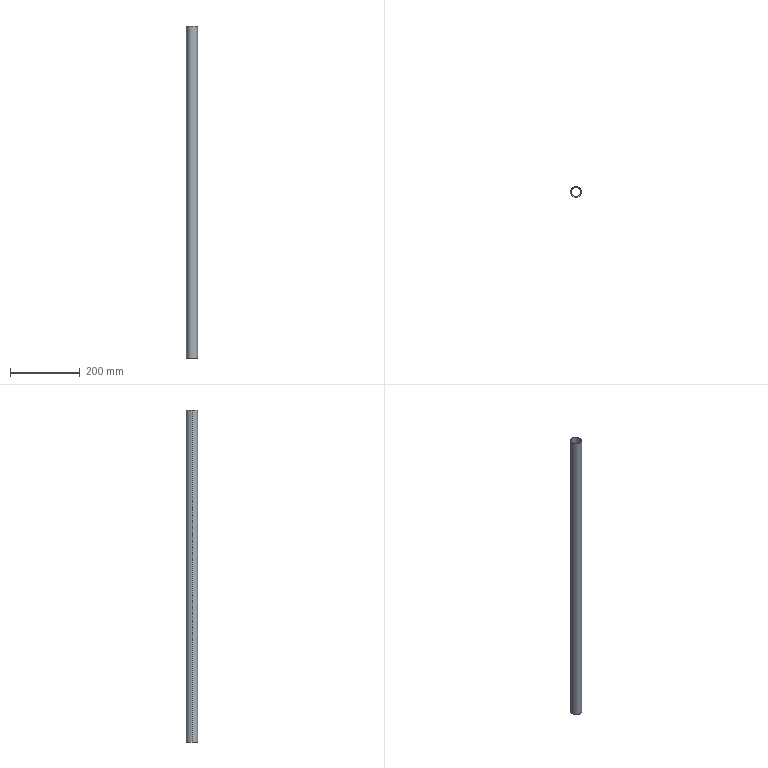Part | SolidWorks | features Extrusion 1 | 1 solid | 6 faces | box 32 x 32 x 950 mm | volume 179071 mm3 | cylinder 4 | plane 2 | commonest cylinder face diameters 28 x2 32 x2
STEP:
#1=CARTESIAN_POINT('',(-14.,0.,475.));
#2=VERTEX_POINT('',#1);
#3=CARTESIAN_POINT('',(14.,0.,475.));
#4=VERTEX_POINT('',#3);
#5=CARTESIAN_POINT('',(0.,0.,475.));
#6=DIRECTION('',(0.,0.,1.));
#7=DIRECTION('',(1.,0.,0.));
#8=AXIS2_PLACEMENT_3D('',#5,#6,#7);
#9=CIRCLE('',#8,14.);
#10=EDGE_CURVE('',#2,#4,#9,.T.);
#11=ORIENTED_EDGE('',*,*,#10,.T.);
#12=CARTESIAN_POINT('',(14.,0.,-475.));
#13=VERTEX_POINT('',#12);
#14=CARTESIAN_POINT('',(14.,0.,475.));
#15=DIRECTION('',(0.,0.,-1.));
#16=VECTOR('',#15,1000.);
#17=LINE('',#14,#16);
#18=EDGE_CURVE('',#4,#13,#17,.T.);
#19=ORIENTED_EDGE('',*,*,#18,.T.);
#20=CARTESIAN_POINT('',(-14.,0.,-475.));
#21=VERTEX_POINT('',#20);
#22=CARTESIAN_POINT('',(0.,0.,-475.));
#23=DIRECTION('',(0.,0.,1.));
#24=DIRECTION('',(1.,0.,0.));
#25=AXIS2_PLACEMENT_3D('',#22,#23,#24);
#26=CIRCLE('',#25,14.);
#27=EDGE_CURVE('',#21,#13,#26,.T.);
#28=ORIENTED_EDGE('',*,*,#27,.F.);
#29=CARTESIAN_POINT('',(-14.,0.,475.));
#30=DIRECTION('',(0.,0.,-1.));
#31=VECTOR('',#30,1000.);
#32=LINE('',#29,#31);
#33=EDGE_CURVE('',#2,#21,#32,.T.);
#34=ORIENTED_EDGE('',*,*,#33,.F.);
#35=EDGE_LOOP('',(#11,#19,#28,#34));
#36=FACE_OUTER_BOUND('',#35,.T.);
#37=CARTESIAN_POINT('',(0.,0.,475.));
#38=DIRECTION('',(0.,0.,-1.));
#39=DIRECTION('',(-1.,0.,0.));
#40=AXIS2_PLACEMENT_3D('',#37,#38,#39);
#41=CYLINDRICAL_SURFACE('',#40,14.);
#42=ADVANCED_FACE('',(#36),#41,.F.);
#43=CARTESIAN_POINT('',(16.,0.,475.));
#44=VERTEX_POINT('',#43);
#45=CARTESIAN_POINT('',(-16.,0.,475.));
#46=VERTEX_POINT('',#45);
#47=CARTESIAN_POINT('',(0.,0.,475.));
#48=DIRECTION('',(0.,0.,1.));
#49=DIRECTION('',(1.,0.,0.));
#50=AXIS2_PLACEMENT_3D('',#47,#48,#49);
#51=CIRCLE('',#50,16.);
#52=EDGE_CURVE('',#44,#46,#51,.T.);
#53=ORIENTED_EDGE('',*,*,#52,.F.);
#54=CARTESIAN_POINT('',(16.,0.,-475.));
#55=VERTEX_POINT('',#54);
#56=CARTESIAN_POINT('',(16.,0.,475.));
#57=DIRECTION('',(0.,0.,-1.));
#58=VECTOR('',#57,1000.);
#59=LINE('',#56,#58);
#60=EDGE_CURVE('',#44,#55,#59,.T.);
#61=ORIENTED_EDGE('',*,*,#60,.T.);
#62=CARTESIAN_POINT('',(-16.,0.,-475.));
#63=VERTEX_POINT('',#62);
#64=CARTESIAN_POINT('',(0.,0.,-475.));
#65=DIRECTION('',(0.,0.,1.));
#66=DIRECTION('',(1.,0.,0.));
#67=AXIS2_PLACEMENT_3D('',#64,#65,#66);
#68=CIRCLE('',#67,16.);
#69=EDGE_CURVE('',#55,#63,#68,.T.);
#70=ORIENTED_EDGE('',*,*,#69,.T.);
#71=CARTESIAN_POINT('',(-16.,0.,475.));
#72=DIRECTION('',(0.,0.,-1.));
#73=VECTOR('',#72,1000.);
#74=LINE('',#71,#73);
#75=EDGE_CURVE('',#46,#63,#74,.T.);
#76=ORIENTED_EDGE('',*,*,#75,.F.);
#77=EDGE_LOOP('',(#53,#61,#70,#76));
#78=FACE_OUTER_BOUND('',#77,.T.);
#79=CARTESIAN_POINT('',(0.,0.,475.));
#80=DIRECTION('',(0.,0.,-1.));
#81=DIRECTION('',(-1.,0.,0.));
#82=AXIS2_PLACEMENT_3D('',#79,#80,#81);
#83=CYLINDRICAL_SURFACE('',#82,16.);
#84=ADVANCED_FACE('',(#78),#83,.T.);
#85=CARTESIAN_POINT('',(0.,0.,475.));
#86=DIRECTION('',(0.,0.,1.));
#87=DIRECTION('',(1.,0.,0.));
#88=AXIS2_PLACEMENT_3D('',#85,#86,#87);
#89=CIRCLE('',#88,16.);
#90=EDGE_CURVE('',#46,#44,#89,.T.);
#91=ORIENTED_EDGE('',*,*,#90,.T.);
#92=ORIENTED_EDGE('',*,*,#52,.T.);
#93=EDGE_LOOP('',(#91,#92));
#94=FACE_OUTER_BOUND('',#93,.T.);
#95=ORIENTED_EDGE('',*,*,#10,.F.);
#96=CARTESIAN_POINT('',(0.,0.,475.));
#97=DIRECTION('',(0.,0.,1.));
#98=DIRECTION('',(1.,0.,0.));
#99=AXIS2_PLACEMENT_3D('',#96,#97,#98);
#100=CIRCLE('',#99,14.);
#101=EDGE_CURVE('',#4,#2,#100,.T.);
#102=ORIENTED_EDGE('',*,*,#101,.F.);
#103=EDGE_LOOP('',(#95,#102));
#104=FACE_BOUND('',#103,.T.);
#105=CARTESIAN_POINT('',(0.,0.,475.));
#106=DIRECTION('',(0.,0.,1.));
#107=DIRECTION('',(1.,0.,0.));
#108=AXIS2_PLACEMENT_3D('',#105,#106,#107);
#109=PLANE('',#108);
#110=ADVANCED_FACE('',(#94,#104),#109,.T.);
#111=CARTESIAN_POINT('',(0.,0.,-475.));
#112=DIRECTION('',(0.,0.,1.));
#113=DIRECTION('',(1.,0.,0.));
#114=AXIS2_PLACEMENT_3D('',#111,#112,#113);
#115=CIRCLE('',#114,16.);
#116=EDGE_CURVE('',#63,#55,#115,.T.);
#117=ORIENTED_EDGE('',*,*,#116,.F.);
#118=ORIENTED_EDGE('',*,*,#69,.F.);
#119=EDGE_LOOP('',(#117,#118));
#120=FACE_OUTER_BOUND('',#119,.T.);
#121=ORIENTED_EDGE('',*,*,#27,.T.);
#122=CARTESIAN_POINT('',(0.,0.,-475.));
#123=DIRECTION('',(0.,0.,1.));
#124=DIRECTION('',(1.,0.,0.));
#125=AXIS2_PLACEMENT_3D('',#122,#123,#124);
#126=CIRCLE('',#125,14.);
#127=EDGE_CURVE('',#13,#21,#126,.T.);
#128=ORIENTED_EDGE('',*,*,#127,.T.);
#129=EDGE_LOOP('',(#121,#128));
#130=FACE_BOUND('',#129,.T.);
#131=CARTESIAN_POINT('',(0.,0.,-475.));
#132=DIRECTION('',(0.,0.,1.));
#133=DIRECTION('',(1.,0.,0.));
#134=AXIS2_PLACEMENT_3D('',#131,#132,#133);
#135=PLANE('',#134);
#136=ADVANCED_FACE('',(#120,#130),#135,.F.);
#137=ORIENTED_EDGE('',*,*,#60,.F.);
#138=ORIENTED_EDGE('',*,*,#90,.F.);
#139=ORIENTED_EDGE('',*,*,#75,.T.);
#140=ORIENTED_EDGE('',*,*,#116,.T.);
#141=EDGE_LOOP('',(#137,#138,#139,#140));
#142=FACE_OUTER_BOUND('',#141,.T.);
#143=CARTESIAN_POINT('',(0.,0.,475.));
#144=DIRECTION('',(0.,0.,-1.));
#145=DIRECTION('',(-1.,0.,0.));
#146=AXIS2_PLACEMENT_3D('',#143,#144,#145);
#147=CYLINDRICAL_SURFACE('',#146,16.);
#148=ADVANCED_FACE('',(#142),#147,.T.);
#149=ORIENTED_EDGE('',*,*,#18,.F.);
#150=ORIENTED_EDGE('',*,*,#101,.T.);
#151=ORIENTED_EDGE('',*,*,#33,.T.);
#152=ORIENTED_EDGE('',*,*,#127,.F.);
#153=EDGE_LOOP('',(#149,#150,#151,#152));
#154=FACE_OUTER_BOUND('',#153,.T.);
#155=CARTESIAN_POINT('',(0.,0.,475.));
#156=DIRECTION('',(0.,0.,-1.));
#157=DIRECTION('',(-1.,0.,0.));
#158=AXIS2_PLACEMENT_3D('',#155,#156,#157);
#159=CYLINDRICAL_SURFACE('',#158,14.);
#160=ADVANCED_FACE('',(#154),#159,.F.);
#161=CLOSED_SHELL('',(#42,#84,#110,#136,#148,#160));
#162=MANIFOLD_SOLID_BREP('',#161);
#163=CARTESIAN_POINT('',(0.,0.,0.));
#164=DIRECTION('',(0.,0.,1.));
#165=DIRECTION('',(1.,0.,0.));
#166=AXIS2_PLACEMENT_3D('',#163,#164,#165);
#167=(LENGTH_UNIT()NAMED_UNIT(*)SI_UNIT(.MILLI.,.METRE.));
#168=UNCERTAINTY_MEASURE_WITH_UNIT(LENGTH_MEASURE(0.00001),#167,'','');
#169=(NAMED_UNIT(*)PLANE_ANGLE_UNIT()SI_UNIT($,.RADIAN.));
#170=(NAMED_UNIT(*)SI_UNIT($,.STERADIAN.)SOLID_ANGLE_UNIT());
#171=(GEOMETRIC_REPRESENTATION_CONTEXT(3)GLOBAL_UNCERTAINTY_ASSIGNED_CONTEXT((#168))GLOBAL_UNIT_ASSIGNED_CONTEXT((#167,#169,#170))REPRESENTATION_CONTEXT('',''));
#172=ADVANCED_BREP_SHAPE_REPRESENTATION('',(#162,#166),#171);